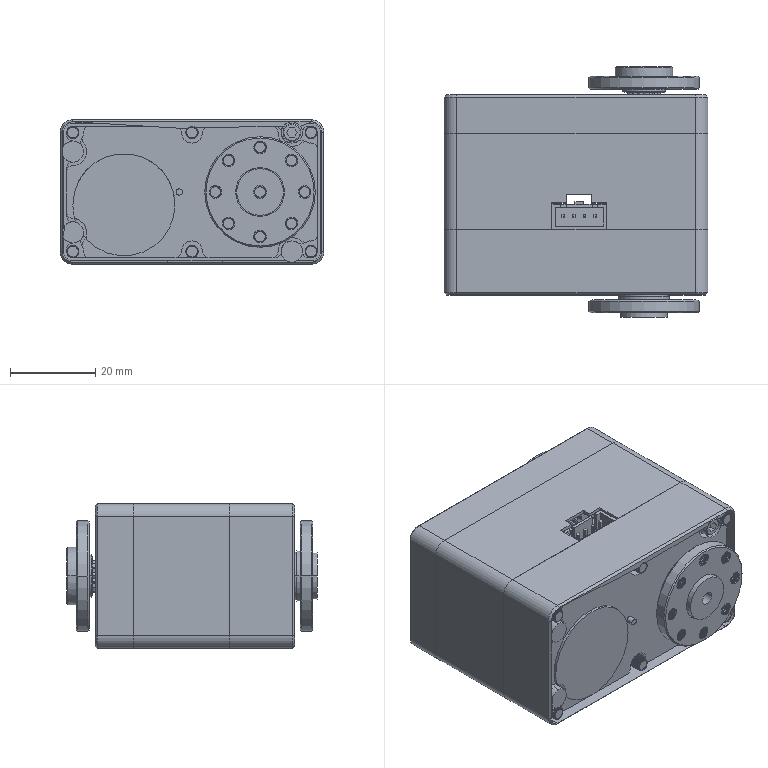Part | NX | features BREP 21 | 21 solids | 3330 faces | volume 1762 mm3 | cylinder 2178 | spline 602 | plane 461 | cone 83 | torus 6 | commonest cylinder face diameters 2.5 x1712 0.38 x88 3 x64 20.55 x44 22.8 x44 1 x32